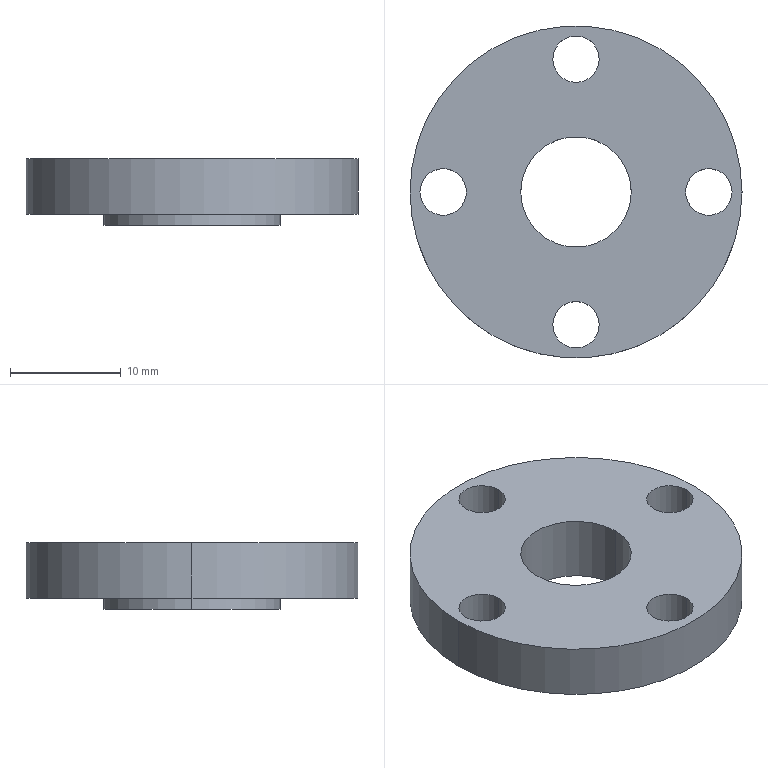Part | SolidWorks | features ICE 3, Chamfer 1, CirPattern 1, Extrusion 1 | 1 solid | 17 faces | box 30 x 30 x 6 mm | volume 2987 mm3 | cylinder 14 | plane 3 | commonest cylinder face diameters 4.2 x8 10 x2 16 x2 30 x2
STEP:
#1=CARTESIAN_POINT('',(-5.,0.,-1.));
#2=VERTEX_POINT('',#1);
#3=CARTESIAN_POINT('',(5.,0.,-1.));
#4=VERTEX_POINT('',#3);
#5=CARTESIAN_POINT('',(0.,0.,-1.));
#6=DIRECTION('',(0.,0.,1.));
#7=DIRECTION('',(1.,0.,0.));
#8=AXIS2_PLACEMENT_3D('',#5,#6,#7);
#9=CIRCLE('',#8,5.);
#10=EDGE_CURVE('',#2,#4,#9,.T.);
#11=ORIENTED_EDGE('',*,*,#10,.F.);
#12=CARTESIAN_POINT('',(-5.,0.,5.));
#13=VERTEX_POINT('',#12);
#14=CARTESIAN_POINT('',(-5.,0.,-1.));
#15=DIRECTION('',(0.,0.,1.));
#16=VECTOR('',#15,1000.);
#17=LINE('',#14,#16);
#18=EDGE_CURVE('',#2,#13,#17,.T.);
#19=ORIENTED_EDGE('',*,*,#18,.T.);
#20=CARTESIAN_POINT('',(5.,0.,5.));
#21=VERTEX_POINT('',#20);
#22=CARTESIAN_POINT('',(0.,0.,5.));
#23=DIRECTION('',(0.,0.,1.));
#24=DIRECTION('',(1.,0.,0.));
#25=AXIS2_PLACEMENT_3D('',#22,#23,#24);
#26=CIRCLE('',#25,5.);
#27=EDGE_CURVE('',#13,#21,#26,.T.);
#28=ORIENTED_EDGE('',*,*,#27,.T.);
#29=CARTESIAN_POINT('',(5.,0.,-1.));
#30=DIRECTION('',(0.,0.,1.));
#31=VECTOR('',#30,1000.);
#32=LINE('',#29,#31);
#33=EDGE_CURVE('',#4,#21,#32,.T.);
#34=ORIENTED_EDGE('',*,*,#33,.F.);
#35=EDGE_LOOP('',(#11,#19,#28,#34));
#36=FACE_OUTER_BOUND('',#35,.T.);
#37=CARTESIAN_POINT('',(0.,0.,-1.));
#38=DIRECTION('',(0.,0.,1.));
#39=DIRECTION('',(1.,0.,0.));
#40=AXIS2_PLACEMENT_3D('',#37,#38,#39);
#41=CYLINDRICAL_SURFACE('',#40,5.);
#42=ADVANCED_FACE('',(#36),#41,.F.);
#43=CARTESIAN_POINT('',(-8.,0.,-1.));
#44=VERTEX_POINT('',#43);
#45=CARTESIAN_POINT('',(8.,0.,-1.));
#46=VERTEX_POINT('',#45);
#47=CARTESIAN_POINT('',(0.,0.,-1.));
#48=DIRECTION('',(0.,0.,-1.));
#49=DIRECTION('',(-1.,0.,0.));
#50=AXIS2_PLACEMENT_3D('',#47,#48,#49);
#51=CIRCLE('',#50,8.);
#52=EDGE_CURVE('',#44,#46,#51,.T.);
#53=ORIENTED_EDGE('',*,*,#52,.F.);
#54=CARTESIAN_POINT('',(-8.,0.,0.));
#55=VERTEX_POINT('',#54);
#56=CARTESIAN_POINT('',(-8.,0.,-1.));
#57=DIRECTION('',(0.,0.,1.));
#58=VECTOR('',#57,1000.);
#59=LINE('',#56,#58);
#60=EDGE_CURVE('',#44,#55,#59,.T.);
#61=ORIENTED_EDGE('',*,*,#60,.T.);
#62=CARTESIAN_POINT('',(8.,0.,0.));
#63=VERTEX_POINT('',#62);
#64=CARTESIAN_POINT('',(0.,0.,0.));
#65=DIRECTION('',(0.,0.,-1.));
#66=DIRECTION('',(1.,0.,0.));
#67=AXIS2_PLACEMENT_3D('',#64,#65,#66);
#68=CIRCLE('',#67,8.);
#69=EDGE_CURVE('',#55,#63,#68,.T.);
#70=ORIENTED_EDGE('',*,*,#69,.T.);
#71=CARTESIAN_POINT('',(8.,0.,-1.));
#72=DIRECTION('',(0.,0.,1.));
#73=VECTOR('',#72,1000.);
#74=LINE('',#71,#73);
#75=EDGE_CURVE('',#46,#63,#74,.T.);
#76=ORIENTED_EDGE('',*,*,#75,.F.);
#77=EDGE_LOOP('',(#53,#61,#70,#76));
#78=FACE_OUTER_BOUND('',#77,.T.);
#79=CARTESIAN_POINT('',(0.,0.,-1.));
#80=DIRECTION('',(0.,0.,1.));
#81=DIRECTION('',(1.,0.,0.));
#82=AXIS2_PLACEMENT_3D('',#79,#80,#81);
#83=CYLINDRICAL_SURFACE('',#82,8.);
#84=ADVANCED_FACE('',(#78),#83,.T.);
#85=CARTESIAN_POINT('',(9.9,0.,0.));
#86=VERTEX_POINT('',#85);
#87=CARTESIAN_POINT('',(14.1,0.,0.));
#88=VERTEX_POINT('',#87);
#89=CARTESIAN_POINT('',(12.,0.,0.));
#90=DIRECTION('',(0.,0.,1.));
#91=DIRECTION('',(0.,-1.,0.));
#92=AXIS2_PLACEMENT_3D('',#89,#90,#91);
#93=CIRCLE('',#92,2.1);
#94=EDGE_CURVE('',#86,#88,#93,.T.);
#95=ORIENTED_EDGE('',*,*,#94,.F.);
#96=CARTESIAN_POINT('',(9.9,0.,5.));
#97=VERTEX_POINT('',#96);
#98=CARTESIAN_POINT('',(9.9,0.,0.));
#99=DIRECTION('',(0.,0.,1.));
#100=VECTOR('',#99,1000.);
#101=LINE('',#98,#100);
#102=EDGE_CURVE('',#86,#97,#101,.T.);
#103=ORIENTED_EDGE('',*,*,#102,.T.);
#104=CARTESIAN_POINT('',(14.1,0.,5.));
#105=VERTEX_POINT('',#104);
#106=CARTESIAN_POINT('',(12.,0.,5.));
#107=DIRECTION('',(0.,0.,1.));
#108=DIRECTION('',(0.,-1.,0.));
#109=AXIS2_PLACEMENT_3D('',#106,#107,#108);
#110=CIRCLE('',#109,2.1);
#111=EDGE_CURVE('',#97,#105,#110,.T.);
#112=ORIENTED_EDGE('',*,*,#111,.T.);
#113=CARTESIAN_POINT('',(14.1,0.,0.));
#114=DIRECTION('',(0.,0.,1.));
#115=VECTOR('',#114,1000.);
#116=LINE('',#113,#115);
#117=EDGE_CURVE('',#88,#105,#116,.T.);
#118=ORIENTED_EDGE('',*,*,#117,.F.);
#119=EDGE_LOOP('',(#95,#103,#112,#118));
#120=FACE_OUTER_BOUND('',#119,.T.);
#121=CARTESIAN_POINT('',(12.,0.,0.));
#122=DIRECTION('',(0.,0.,1.));
#123=DIRECTION('',(1.,0.,0.));
#124=AXIS2_PLACEMENT_3D('',#121,#122,#123);
#125=CYLINDRICAL_SURFACE('',#124,2.1);
#126=ADVANCED_FACE('',(#120),#125,.F.);
#127=CARTESIAN_POINT('',(-2.1,-12.,0.));
#128=VERTEX_POINT('',#127);
#129=CARTESIAN_POINT('',(2.1,-12.,0.));
#130=VERTEX_POINT('',#129);
#131=CARTESIAN_POINT('',(0.,-12.,0.));
#132=DIRECTION('',(0.,0.,1.));
#133=DIRECTION('',(-1.,0.,0.));
#134=AXIS2_PLACEMENT_3D('',#131,#132,#133);
#135=CIRCLE('',#134,2.1);
#136=EDGE_CURVE('',#128,#130,#135,.T.);
#137=ORIENTED_EDGE('',*,*,#136,.F.);
#138=CARTESIAN_POINT('',(-2.1,-12.,5.));
#139=VERTEX_POINT('',#138);
#140=CARTESIAN_POINT('',(-2.1,-12.,0.));
#141=DIRECTION('',(0.,0.,1.));
#142=VECTOR('',#141,1000.);
#143=LINE('',#140,#142);
#144=EDGE_CURVE('',#128,#139,#143,.T.);
#145=ORIENTED_EDGE('',*,*,#144,.T.);
#146=CARTESIAN_POINT('',(2.1,-12.,5.));
#147=VERTEX_POINT('',#146);
#148=CARTESIAN_POINT('',(0.,-12.,5.));
#149=DIRECTION('',(0.,0.,1.));
#150=DIRECTION('',(-1.,0.,0.));
#151=AXIS2_PLACEMENT_3D('',#148,#149,#150);
#152=CIRCLE('',#151,2.1);
#153=EDGE_CURVE('',#139,#147,#152,.T.);
#154=ORIENTED_EDGE('',*,*,#153,.T.);
#155=CARTESIAN_POINT('',(2.1,-12.,0.));
#156=DIRECTION('',(0.,0.,1.));
#157=VECTOR('',#156,1000.);
#158=LINE('',#155,#157);
#159=EDGE_CURVE('',#130,#147,#158,.T.);
#160=ORIENTED_EDGE('',*,*,#159,.F.);
#161=EDGE_LOOP('',(#137,#145,#154,#160));
#162=FACE_OUTER_BOUND('',#161,.T.);
#163=CARTESIAN_POINT('',(0.,-12.,0.));
#164=DIRECTION('',(0.,0.,1.));
#165=DIRECTION('',(1.,0.,0.));
#166=AXIS2_PLACEMENT_3D('',#163,#164,#165);
#167=CYLINDRICAL_SURFACE('',#166,2.1);
#168=ADVANCED_FACE('',(#162),#167,.F.);
#169=CARTESIAN_POINT('',(-14.1,0.,0.));
#170=VERTEX_POINT('',#169);
#171=CARTESIAN_POINT('',(-9.9,0.,0.));
#172=VERTEX_POINT('',#171);
#173=CARTESIAN_POINT('',(-12.,0.,0.));
#174=DIRECTION('',(0.,0.,1.));
#175=DIRECTION('',(0.,1.,0.));
#176=AXIS2_PLACEMENT_3D('',#173,#174,#175);
#177=CIRCLE('',#176,2.1);
#178=EDGE_CURVE('',#170,#172,#177,.T.);
#179=ORIENTED_EDGE('',*,*,#178,.F.);
#180=CARTESIAN_POINT('',(-14.1,0.,5.));
#181=VERTEX_POINT('',#180);
#182=CARTESIAN_POINT('',(-14.1,0.,0.));
#183=DIRECTION('',(0.,0.,1.));
#184=VECTOR('',#183,1000.);
#185=LINE('',#182,#184);
#186=EDGE_CURVE('',#170,#181,#185,.T.);
#187=ORIENTED_EDGE('',*,*,#186,.T.);
#188=CARTESIAN_POINT('',(-9.9,0.,5.));
#189=VERTEX_POINT('',#188);
#190=CARTESIAN_POINT('',(-12.,0.,5.));
#191=DIRECTION('',(0.,0.,1.));
#192=DIRECTION('',(0.,1.,0.));
#193=AXIS2_PLACEMENT_3D('',#190,#191,#192);
#194=CIRCLE('',#193,2.1);
#195=EDGE_CURVE('',#181,#189,#194,.T.);
#196=ORIENTED_EDGE('',*,*,#195,.T.);
#197=CARTESIAN_POINT('',(-9.9,0.,0.));
#198=DIRECTION('',(0.,0.,1.));
#199=VECTOR('',#198,1000.);
#200=LINE('',#197,#199);
#201=EDGE_CURVE('',#172,#189,#200,.T.);
#202=ORIENTED_EDGE('',*,*,#201,.F.);
#203=EDGE_LOOP('',(#179,#187,#196,#202));
#204=FACE_OUTER_BOUND('',#203,.T.);
#205=CARTESIAN_POINT('',(-12.,0.,0.));
#206=DIRECTION('',(0.,0.,1.));
#207=DIRECTION('',(1.,0.,0.));
#208=AXIS2_PLACEMENT_3D('',#205,#206,#207);
#209=CYLINDRICAL_SURFACE('',#208,2.1);
#210=ADVANCED_FACE('',(#204),#209,.F.);
#211=CARTESIAN_POINT('',(-2.1,12.,0.));
#212=VERTEX_POINT('',#211);
#213=CARTESIAN_POINT('',(2.1,12.,0.));
#214=VERTEX_POINT('',#213);
#215=CARTESIAN_POINT('',(0.,12.,0.));
#216=DIRECTION('',(0.,0.,1.));
#217=DIRECTION('',(1.,0.,0.));
#218=AXIS2_PLACEMENT_3D('',#215,#216,#217);
#219=CIRCLE('',#218,2.1);
#220=EDGE_CURVE('',#212,#214,#219,.T.);
#221=ORIENTED_EDGE('',*,*,#220,.F.);
#222=CARTESIAN_POINT('',(-2.1,12.,5.));
#223=VERTEX_POINT('',#222);
#224=CARTESIAN_POINT('',(-2.1,12.,0.));
#225=DIRECTION('',(0.,0.,1.));
#226=VECTOR('',#225,1000.);
#227=LINE('',#224,#226);
#228=EDGE_CURVE('',#212,#223,#227,.T.);
#229=ORIENTED_EDGE('',*,*,#228,.T.);
#230=CARTESIAN_POINT('',(2.1,12.,5.));
#231=VERTEX_POINT('',#230);
#232=CARTESIAN_POINT('',(0.,12.,5.));
#233=DIRECTION('',(0.,0.,1.));
#234=DIRECTION('',(1.,0.,0.));
#235=AXIS2_PLACEMENT_3D('',#232,#233,#234);
#236=CIRCLE('',#235,2.1);
#237=EDGE_CURVE('',#223,#231,#236,.T.);
#238=ORIENTED_EDGE('',*,*,#237,.T.);
#239=CARTESIAN_POINT('',(2.1,12.,0.));
#240=DIRECTION('',(0.,0.,1.));
#241=VECTOR('',#240,1000.);
#242=LINE('',#239,#241);
#243=EDGE_CURVE('',#214,#231,#242,.T.);
#244=ORIENTED_EDGE('',*,*,#243,.F.);
#245=EDGE_LOOP('',(#221,#229,#238,#244));
#246=FACE_OUTER_BOUND('',#245,.T.);
#247=CARTESIAN_POINT('',(0.,12.,0.));
#248=DIRECTION('',(0.,0.,1.));
#249=DIRECTION('',(1.,0.,0.));
#250=AXIS2_PLACEMENT_3D('',#247,#248,#249);
#251=CYLINDRICAL_SURFACE('',#250,2.1);
#252=ADVANCED_FACE('',(#246),#251,.F.);
#253=CARTESIAN_POINT('',(15.,0.,5.));
#254=VERTEX_POINT('',#253);
#255=CARTESIAN_POINT('',(-15.,0.,5.));
#256=VERTEX_POINT('',#255);
#257=CARTESIAN_POINT('',(0.,0.,5.));
#258=DIRECTION('',(0.,0.,1.));
#259=DIRECTION('',(1.,0.,0.));
#260=AXIS2_PLACEMENT_3D('',#257,#258,#259);
#261=CIRCLE('',#260,15.);
#262=EDGE_CURVE('',#254,#256,#261,.T.);
#263=ORIENTED_EDGE('',*,*,#262,.F.);
#264=CARTESIAN_POINT('',(15.,0.,0.));
#265=VERTEX_POINT('',#264);
#266=CARTESIAN_POINT('',(15.,0.,5.));
#267=DIRECTION('',(0.,0.,-1.));
#268=VECTOR('',#267,1000.);
#269=LINE('',#266,#268);
#270=EDGE_CURVE('',#254,#265,#269,.T.);
#271=ORIENTED_EDGE('',*,*,#270,.T.);
#272=CARTESIAN_POINT('',(-15.,0.,0.));
#273=VERTEX_POINT('',#272);
#274=CARTESIAN_POINT('',(0.,0.,0.));
#275=DIRECTION('',(0.,0.,1.));
#276=DIRECTION('',(1.,0.,0.));
#277=AXIS2_PLACEMENT_3D('',#274,#275,#276);
#278=CIRCLE('',#277,15.);
#279=EDGE_CURVE('',#265,#273,#278,.T.);
#280=ORIENTED_EDGE('',*,*,#279,.T.);
#281=CARTESIAN_POINT('',(-15.,0.,5.));
#282=DIRECTION('',(0.,0.,-1.));
#283=VECTOR('',#282,1000.);
#284=LINE('',#281,#283);
#285=EDGE_CURVE('',#256,#273,#284,.T.);
#286=ORIENTED_EDGE('',*,*,#285,.F.);
#287=EDGE_LOOP('',(#263,#271,#280,#286));
#288=FACE_OUTER_BOUND('',#287,.T.);
#289=CARTESIAN_POINT('',(0.,0.,5.));
#290=DIRECTION('',(0.,0.,-1.));
#291=DIRECTION('',(-1.,0.,0.));
#292=AXIS2_PLACEMENT_3D('',#289,#290,#291);
#293=CYLINDRICAL_SURFACE('',#292,15.);
#294=ADVANCED_FACE('',(#288),#293,.T.);
#295=ORIENTED_EDGE('',*,*,#270,.F.);
#296=CARTESIAN_POINT('',(0.,0.,5.));
#297=DIRECTION('',(0.,0.,1.));
#298=DIRECTION('',(1.,0.,0.));
#299=AXIS2_PLACEMENT_3D('',#296,#297,#298);
#300=CIRCLE('',#299,15.);
#301=EDGE_CURVE('',#256,#254,#300,.T.);
#302=ORIENTED_EDGE('',*,*,#301,.F.);
#303=ORIENTED_EDGE('',*,*,#285,.T.);
#304=CARTESIAN_POINT('',(0.,0.,0.));
#305=DIRECTION('',(0.,0.,1.));
#306=DIRECTION('',(1.,0.,0.));
#307=AXIS2_PLACEMENT_3D('',#304,#305,#306);
#308=CIRCLE('',#307,15.);
#309=EDGE_CURVE('',#273,#265,#308,.T.);
#310=ORIENTED_EDGE('',*,*,#309,.T.);
#311=EDGE_LOOP('',(#295,#302,#303,#310));
#312=FACE_OUTER_BOUND('',#311,.T.);
#313=CARTESIAN_POINT('',(0.,0.,5.));
#314=DIRECTION('',(0.,0.,-1.));
#315=DIRECTION('',(-1.,0.,0.));
#316=AXIS2_PLACEMENT_3D('',#313,#314,#315);
#317=CYLINDRICAL_SURFACE('',#316,15.);
#318=ADVANCED_FACE('',(#312),#317,.T.);
#319=CARTESIAN_POINT('',(0.,0.,5.));
#320=DIRECTION('',(0.,0.,1.));
#321=DIRECTION('',(1.,0.,0.));
#322=AXIS2_PLACEMENT_3D('',#319,#320,#321);
#323=CIRCLE('',#322,5.);
#324=EDGE_CURVE('',#21,#13,#323,.T.);
#325=ORIENTED_EDGE('',*,*,#324,.F.);
#326=ORIENTED_EDGE('',*,*,#27,.F.);
#327=EDGE_LOOP('',(#325,#326));
#328=FACE_BOUND('',#327,.T.);
#329=CARTESIAN_POINT('',(12.,0.,5.));
#330=DIRECTION('',(0.,0.,1.));
#331=DIRECTION('',(0.,-1.,0.));
#332=AXIS2_PLACEMENT_3D('',#329,#330,#331);
#333=CIRCLE('',#332,2.1);
#334=EDGE_CURVE('',#105,#97,#333,.T.);
#335=ORIENTED_EDGE('',*,*,#334,.F.);
#336=ORIENTED_EDGE('',*,*,#111,.F.);
#337=EDGE_LOOP('',(#335,#336));
#338=FACE_BOUND('',#337,.T.);
#339=CARTESIAN_POINT('',(0.,-12.,5.));
#340=DIRECTION('',(0.,0.,1.));
#341=DIRECTION('',(-1.,0.,0.));
#342=AXIS2_PLACEMENT_3D('',#339,#340,#341);
#343=CIRCLE('',#342,2.1);
#344=EDGE_CURVE('',#147,#139,#343,.T.);
#345=ORIENTED_EDGE('',*,*,#344,.F.);
#346=ORIENTED_EDGE('',*,*,#153,.F.);
#347=EDGE_LOOP('',(#345,#346));
#348=FACE_BOUND('',#347,.T.);
#349=CARTESIAN_POINT('',(-12.,0.,5.));
#350=DIRECTION('',(0.,0.,1.));
#351=DIRECTION('',(0.,1.,0.));
#352=AXIS2_PLACEMENT_3D('',#349,#350,#351);
#353=CIRCLE('',#352,2.1);
#354=EDGE_CURVE('',#189,#181,#353,.T.);
#355=ORIENTED_EDGE('',*,*,#354,.F.);
#356=ORIENTED_EDGE('',*,*,#195,.F.);
#357=EDGE_LOOP('',(#355,#356));
#358=FACE_BOUND('',#357,.T.);
#359=CARTESIAN_POINT('',(0.,12.,5.));
#360=DIRECTION('',(0.,0.,1.));
#361=DIRECTION('',(1.,0.,0.));
#362=AXIS2_PLACEMENT_3D('',#359,#360,#361);
#363=CIRCLE('',#362,2.1);
#364=EDGE_CURVE('',#231,#223,#363,.T.);
#365=ORIENTED_EDGE('',*,*,#364,.F.);
#366=ORIENTED_EDGE('',*,*,#237,.F.);
#367=EDGE_LOOP('',(#365,#366));
#368=FACE_BOUND('',#367,.T.);
#369=ORIENTED_EDGE('',*,*,#301,.T.);
#370=ORIENTED_EDGE('',*,*,#262,.T.);
#371=EDGE_LOOP('',(#369,#370));
#372=FACE_OUTER_BOUND('',#371,.T.);
#373=CARTESIAN_POINT('',(0.,0.,5.));
#374=DIRECTION('',(0.,0.,1.));
#375=DIRECTION('',(1.,0.,0.));
#376=AXIS2_PLACEMENT_3D('',#373,#374,#375);
#377=PLANE('',#376);
#378=ADVANCED_FACE('',(#328,#338,#348,#358,#368,#372),#377,.T.);
#379=CARTESIAN_POINT('',(0.,0.,0.));
#380=DIRECTION('',(0.,0.,-1.));
#381=DIRECTION('',(1.,0.,0.));
#382=AXIS2_PLACEMENT_3D('',#379,#380,#381);
#383=CIRCLE('',#382,8.);
#384=EDGE_CURVE('',#63,#55,#383,.T.);
#385=ORIENTED_EDGE('',*,*,#384,.F.);
#386=ORIENTED_EDGE('',*,*,#69,.F.);
#387=EDGE_LOOP('',(#385,#386));
#388=FACE_BOUND('',#387,.T.);
#389=CARTESIAN_POINT('',(12.,0.,0.));
#390=DIRECTION('',(0.,0.,1.));
#391=DIRECTION('',(0.,-1.,0.));
#392=AXIS2_PLACEMENT_3D('',#389,#390,#391);
#393=CIRCLE('',#392,2.1);
#394=EDGE_CURVE('',#88,#86,#393,.T.);
#395=ORIENTED_EDGE('',*,*,#394,.T.);
#396=ORIENTED_EDGE('',*,*,#94,.T.);
#397=EDGE_LOOP('',(#395,#396));
#398=FACE_BOUND('',#397,.T.);
#399=CARTESIAN_POINT('',(0.,-12.,0.));
#400=DIRECTION('',(0.,0.,1.));
#401=DIRECTION('',(-1.,0.,0.));
#402=AXIS2_PLACEMENT_3D('',#399,#400,#401);
#403=CIRCLE('',#402,2.1);
#404=EDGE_CURVE('',#130,#128,#403,.T.);
#405=ORIENTED_EDGE('',*,*,#404,.T.);
#406=ORIENTED_EDGE('',*,*,#136,.T.);
#407=EDGE_LOOP('',(#405,#406));
#408=FACE_BOUND('',#407,.T.);
#409=CARTESIAN_POINT('',(-12.,0.,0.));
#410=DIRECTION('',(0.,0.,1.));
#411=DIRECTION('',(0.,1.,0.));
#412=AXIS2_PLACEMENT_3D('',#409,#410,#411);
#413=CIRCLE('',#412,2.1);
#414=EDGE_CURVE('',#172,#170,#413,.T.);
#415=ORIENTED_EDGE('',*,*,#414,.T.);
#416=ORIENTED_EDGE('',*,*,#178,.T.);
#417=EDGE_LOOP('',(#415,#416));
#418=FACE_BOUND('',#417,.T.);
#419=CARTESIAN_POINT('',(0.,12.,0.));
#420=DIRECTION('',(0.,0.,1.));
#421=DIRECTION('',(1.,0.,0.));
#422=AXIS2_PLACEMENT_3D('',#419,#420,#421);
#423=CIRCLE('',#422,2.1);
#424=EDGE_CURVE('',#214,#212,#423,.T.);
#425=ORIENTED_EDGE('',*,*,#424,.T.);
#426=ORIENTED_EDGE('',*,*,#220,.T.);
#427=EDGE_LOOP('',(#425,#426));
#428=FACE_BOUND('',#427,.T.);
#429=ORIENTED_EDGE('',*,*,#309,.F.);
#430=ORIENTED_EDGE('',*,*,#279,.F.);
#431=EDGE_LOOP('',(#429,#430));
#432=FACE_OUTER_BOUND('',#431,.T.);
#433=CARTESIAN_POINT('',(0.,0.,0.));
#434=DIRECTION('',(0.,0.,1.));
#435=DIRECTION('',(1.,0.,0.));
#436=AXIS2_PLACEMENT_3D('',#433,#434,#435);
#437=PLANE('',#436);
#438=ADVANCED_FACE('',(#388,#398,#408,#418,#428,#432),#437,.F.);
#439=ORIENTED_EDGE('',*,*,#228,.F.);
#440=ORIENTED_EDGE('',*,*,#424,.F.);
#441=ORIENTED_EDGE('',*,*,#243,.T.);
#442=ORIENTED_EDGE('',*,*,#364,.T.);
#443=EDGE_LOOP('',(#439,#440,#441,#442));
#444=FACE_OUTER_BOUND('',#443,.T.);
#445=CARTESIAN_POINT('',(0.,12.,0.));
#446=DIRECTION('',(0.,0.,1.));
#447=DIRECTION('',(1.,0.,0.));
#448=AXIS2_PLACEMENT_3D('',#445,#446,#447);
#449=CYLINDRICAL_SURFACE('',#448,2.1);
#450=ADVANCED_FACE('',(#444),#449,.F.);
#451=ORIENTED_EDGE('',*,*,#186,.F.);
#452=ORIENTED_EDGE('',*,*,#414,.F.);
#453=ORIENTED_EDGE('',*,*,#201,.T.);
#454=ORIENTED_EDGE('',*,*,#354,.T.);
#455=EDGE_LOOP('',(#451,#452,#453,#454));
#456=FACE_OUTER_BOUND('',#455,.T.);
#457=CARTESIAN_POINT('',(-12.,0.,0.));
#458=DIRECTION('',(0.,0.,1.));
#459=DIRECTION('',(1.,0.,0.));
#460=AXIS2_PLACEMENT_3D('',#457,#458,#459);
#461=CYLINDRICAL_SURFACE('',#460,2.1);
#462=ADVANCED_FACE('',(#456),#461,.F.);
#463=ORIENTED_EDGE('',*,*,#144,.F.);
#464=ORIENTED_EDGE('',*,*,#404,.F.);
#465=ORIENTED_EDGE('',*,*,#159,.T.);
#466=ORIENTED_EDGE('',*,*,#344,.T.);
#467=EDGE_LOOP('',(#463,#464,#465,#466));
#468=FACE_OUTER_BOUND('',#467,.T.);
#469=CARTESIAN_POINT('',(0.,-12.,0.));
#470=DIRECTION('',(0.,0.,1.));
#471=DIRECTION('',(1.,0.,0.));
#472=AXIS2_PLACEMENT_3D('',#469,#470,#471);
#473=CYLINDRICAL_SURFACE('',#472,2.1);
#474=ADVANCED_FACE('',(#468),#473,.F.);
#475=ORIENTED_EDGE('',*,*,#102,.F.);
#476=ORIENTED_EDGE('',*,*,#394,.F.);
#477=ORIENTED_EDGE('',*,*,#117,.T.);
#478=ORIENTED_EDGE('',*,*,#334,.T.);
#479=EDGE_LOOP('',(#475,#476,#477,#478));
#480=FACE_OUTER_BOUND('',#479,.T.);
#481=CARTESIAN_POINT('',(12.,0.,0.));
#482=DIRECTION('',(0.,0.,1.));
#483=DIRECTION('',(1.,0.,0.));
#484=AXIS2_PLACEMENT_3D('',#481,#482,#483);
#485=CYLINDRICAL_SURFACE('',#484,2.1);
#486=ADVANCED_FACE('',(#480),#485,.F.);
#487=ORIENTED_EDGE('',*,*,#60,.F.);
#488=CARTESIAN_POINT('',(0.,0.,-1.));
#489=DIRECTION('',(0.,0.,-1.));
#490=DIRECTION('',(-1.,0.,0.));
#491=AXIS2_PLACEMENT_3D('',#488,#489,#490);
#492=CIRCLE('',#491,8.);
#493=EDGE_CURVE('',#46,#44,#492,.T.);
#494=ORIENTED_EDGE('',*,*,#493,.F.);
#495=ORIENTED_EDGE('',*,*,#75,.T.);
#496=ORIENTED_EDGE('',*,*,#384,.T.);
#497=EDGE_LOOP('',(#487,#494,#495,#496));
#498=FACE_OUTER_BOUND('',#497,.T.);
#499=CARTESIAN_POINT('',(0.,0.,-1.));
#500=DIRECTION('',(0.,0.,1.));
#501=DIRECTION('',(1.,0.,0.));
#502=AXIS2_PLACEMENT_3D('',#499,#500,#501);
#503=CYLINDRICAL_SURFACE('',#502,8.);
#504=ADVANCED_FACE('',(#498),#503,.T.);
#505=CARTESIAN_POINT('',(0.,0.,-1.));
#506=DIRECTION('',(0.,0.,1.));
#507=DIRECTION('',(1.,0.,0.));
#508=AXIS2_PLACEMENT_3D('',#505,#506,#507);
#509=CIRCLE('',#508,5.);
#510=EDGE_CURVE('',#4,#2,#509,.T.);
#511=ORIENTED_EDGE('',*,*,#510,.T.);
#512=ORIENTED_EDGE('',*,*,#10,.T.);
#513=EDGE_LOOP('',(#511,#512));
#514=FACE_BOUND('',#513,.T.);
#515=ORIENTED_EDGE('',*,*,#493,.T.);
#516=ORIENTED_EDGE('',*,*,#52,.T.);
#517=EDGE_LOOP('',(#515,#516));
#518=FACE_OUTER_BOUND('',#517,.T.);
#519=CARTESIAN_POINT('',(0.,0.,-1.));
#520=DIRECTION('',(0.,0.,-1.));
#521=DIRECTION('',(-1.,0.,0.));
#522=AXIS2_PLACEMENT_3D('',#519,#520,#521);
#523=PLANE('',#522);
#524=ADVANCED_FACE('',(#514,#518),#523,.T.);
#525=ORIENTED_EDGE('',*,*,#18,.F.);
#526=ORIENTED_EDGE('',*,*,#510,.F.);
#527=ORIENTED_EDGE('',*,*,#33,.T.);
#528=ORIENTED_EDGE('',*,*,#324,.T.);
#529=EDGE_LOOP('',(#525,#526,#527,#528));
#530=FACE_OUTER_BOUND('',#529,.T.);
#531=CARTESIAN_POINT('',(0.,0.,-1.));
#532=DIRECTION('',(0.,0.,1.));
#533=DIRECTION('',(1.,0.,0.));
#534=AXIS2_PLACEMENT_3D('',#531,#532,#533);
#535=CYLINDRICAL_SURFACE('',#534,5.);
#536=ADVANCED_FACE('',(#530),#535,.F.);
#537=CLOSED_SHELL('',(#42,#84,#126,#168,#210,#252,#294,#318,#378,#438,#450,#462,#474,#486,#504,#524,#536));
#538=MANIFOLD_SOLID_BREP('',#537);
#539=CARTESIAN_POINT('',(0.,0.,0.));
#540=DIRECTION('',(0.,0.,1.));
#541=DIRECTION('',(1.,0.,0.));
#542=AXIS2_PLACEMENT_3D('',#539,#540,#541);
#543=(LENGTH_UNIT()NAMED_UNIT(*)SI_UNIT(.MILLI.,.METRE.));
#544=UNCERTAINTY_MEASURE_WITH_UNIT(LENGTH_MEASURE(0.00001),#543,'','');
#545=(NAMED_UNIT(*)PLANE_ANGLE_UNIT()SI_UNIT($,.RADIAN.));
#546=(NAMED_UNIT(*)SI_UNIT($,.STERADIAN.)SOLID_ANGLE_UNIT());
#547=(GEOMETRIC_REPRESENTATION_CONTEXT(3)GLOBAL_UNCERTAINTY_ASSIGNED_CONTEXT((#544))GLOBAL_UNIT_ASSIGNED_CONTEXT((#543,#545,#546))REPRESENTATION_CONTEXT('',''));
#548=ADVANCED_BREP_SHAPE_REPRESENTATION('',(#538,#542),#547);